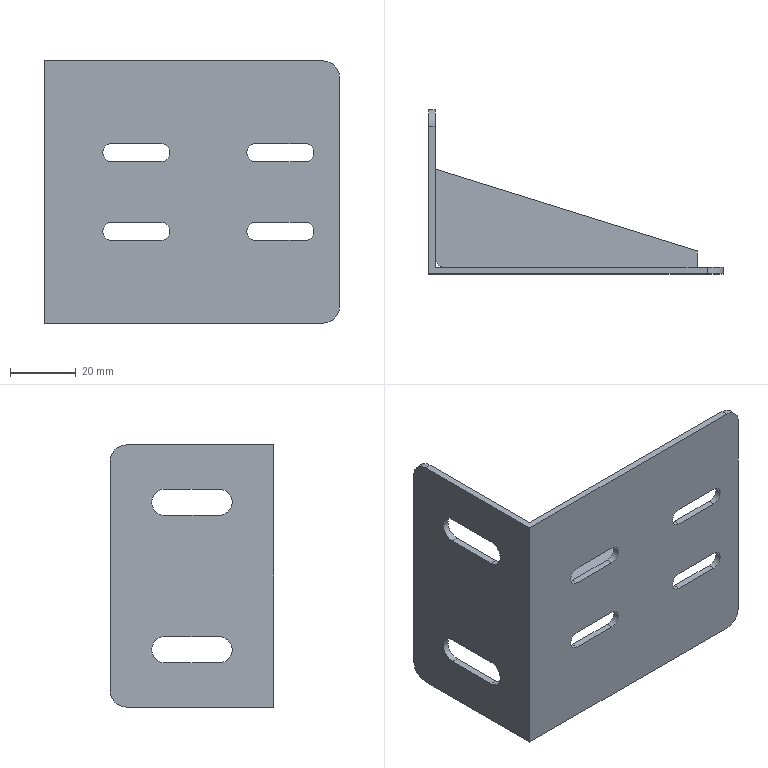Part | SolidWorks | features ICE 3, ExtruThin 1, Fillet 1 | 2 solids | 45 faces | box 90 x 50 x 80 mm | volume 23252 mm3 | plane 26 | cylinder 19 | commonest cylinder face diameters 5.5 x8 8 x6 10 x4 6 x1
STEP:
#1=CARTESIAN_POINT('',(2.,32.,-1.));
#2=VERTEX_POINT('',#1);
#3=CARTESIAN_POINT('',(2.,5.,-1.));
#4=VERTEX_POINT('',#3);
#5=CARTESIAN_POINT('',(2.,5.,-1.));
#6=DIRECTION('',(0.,-1.,0.));
#7=VECTOR('',#6,1000.);
#8=LINE('',#5,#7);
#9=EDGE_CURVE('',#2,#4,#8,.T.);
#10=ORIENTED_EDGE('',*,*,#9,.T.);
#11=CARTESIAN_POINT('',(2.,5.,1.));
#12=VERTEX_POINT('',#11);
#13=CARTESIAN_POINT('',(2.,5.,1.));
#14=DIRECTION('',(0.,0.,-1.));
#15=VECTOR('',#14,1000.);
#16=LINE('',#13,#15);
#17=EDGE_CURVE('',#12,#4,#16,.T.);
#18=ORIENTED_EDGE('',*,*,#17,.F.);
#19=CARTESIAN_POINT('',(2.,32.,1.));
#20=VERTEX_POINT('',#19);
#21=CARTESIAN_POINT('',(2.,5.,1.));
#22=DIRECTION('',(0.,-1.,0.));
#23=VECTOR('',#22,1000.);
#24=LINE('',#21,#23);
#25=EDGE_CURVE('',#20,#12,#24,.T.);
#26=ORIENTED_EDGE('',*,*,#25,.F.);
#27=CARTESIAN_POINT('',(2.,32.,1.));
#28=DIRECTION('',(0.,0.,-1.));
#29=VECTOR('',#28,1000.);
#30=LINE('',#27,#29);
#31=EDGE_CURVE('',#20,#2,#30,.T.);
#32=ORIENTED_EDGE('',*,*,#31,.T.);
#33=EDGE_LOOP('',(#10,#18,#26,#32));
#34=FACE_OUTER_BOUND('',#33,.T.);
#35=CARTESIAN_POINT('',(2.,5.,1.));
#36=DIRECTION('',(1.,0.,0.));
#37=DIRECTION('',(0.,1.,0.));
#38=AXIS2_PLACEMENT_3D('',#35,#36,#37);
#39=PLANE('',#38);
#40=ADVANCED_FACE('',(#34),#39,.F.);
#41=CARTESIAN_POINT('',(5.,2.,-1.));
#42=VERTEX_POINT('',#41);
#43=CARTESIAN_POINT('',(5.,5.,-1.));
#44=DIRECTION('',(0.,0.,1.));
#45=DIRECTION('',(-1.,0.,0.));
#46=AXIS2_PLACEMENT_3D('',#43,#44,#45);
#47=CIRCLE('',#46,3.);
#48=EDGE_CURVE('',#4,#42,#47,.T.);
#49=ORIENTED_EDGE('',*,*,#48,.T.);
#50=CARTESIAN_POINT('',(5.,2.,1.));
#51=VERTEX_POINT('',#50);
#52=CARTESIAN_POINT('',(5.,2.,1.));
#53=DIRECTION('',(0.,0.,-1.));
#54=VECTOR('',#53,1000.);
#55=LINE('',#52,#54);
#56=EDGE_CURVE('',#51,#42,#55,.T.);
#57=ORIENTED_EDGE('',*,*,#56,.F.);
#58=CARTESIAN_POINT('',(5.,5.,1.));
#59=DIRECTION('',(0.,0.,1.));
#60=DIRECTION('',(-1.,0.,0.));
#61=AXIS2_PLACEMENT_3D('',#58,#59,#60);
#62=CIRCLE('',#61,3.);
#63=EDGE_CURVE('',#12,#51,#62,.T.);
#64=ORIENTED_EDGE('',*,*,#63,.F.);
#65=ORIENTED_EDGE('',*,*,#17,.T.);
#66=EDGE_LOOP('',(#49,#57,#64,#65));
#67=FACE_OUTER_BOUND('',#66,.T.);
#68=CARTESIAN_POINT('',(5.,5.,1.));
#69=DIRECTION('',(0.,0.,-1.));
#70=DIRECTION('',(-1.,0.,0.));
#71=AXIS2_PLACEMENT_3D('',#68,#69,#70);
#72=CYLINDRICAL_SURFACE('',#71,3.);
#73=ADVANCED_FACE('',(#67),#72,.T.);
#74=CARTESIAN_POINT('',(82.,2.,-1.));
#75=VERTEX_POINT('',#74);
#76=CARTESIAN_POINT('',(82.,2.,-1.));
#77=DIRECTION('',(1.,0.,0.));
#78=VECTOR('',#77,1000.);
#79=LINE('',#76,#78);
#80=EDGE_CURVE('',#42,#75,#79,.T.);
#81=ORIENTED_EDGE('',*,*,#80,.T.);
#82=CARTESIAN_POINT('',(82.,2.,1.));
#83=VERTEX_POINT('',#82);
#84=CARTESIAN_POINT('',(82.,2.,1.));
#85=DIRECTION('',(0.,0.,-1.));
#86=VECTOR('',#85,1000.);
#87=LINE('',#84,#86);
#88=EDGE_CURVE('',#83,#75,#87,.T.);
#89=ORIENTED_EDGE('',*,*,#88,.F.);
#90=CARTESIAN_POINT('',(82.,2.,1.));
#91=DIRECTION('',(1.,0.,0.));
#92=VECTOR('',#91,1000.);
#93=LINE('',#90,#92);
#94=EDGE_CURVE('',#51,#83,#93,.T.);
#95=ORIENTED_EDGE('',*,*,#94,.F.);
#96=ORIENTED_EDGE('',*,*,#56,.T.);
#97=EDGE_LOOP('',(#81,#89,#95,#96));
#98=FACE_OUTER_BOUND('',#97,.T.);
#99=CARTESIAN_POINT('',(82.,2.,1.));
#100=DIRECTION('',(0.,1.,0.));
#101=DIRECTION('',(0.,0.,1.));
#102=AXIS2_PLACEMENT_3D('',#99,#100,#101);
#103=PLANE('',#102);
#104=ADVANCED_FACE('',(#98),#103,.F.);
#105=CARTESIAN_POINT('',(82.,7.,-1.));
#106=VERTEX_POINT('',#105);
#107=CARTESIAN_POINT('',(82.,7.,-1.));
#108=DIRECTION('',(0.,1.,0.));
#109=VECTOR('',#108,1000.);
#110=LINE('',#107,#109);
#111=EDGE_CURVE('',#75,#106,#110,.T.);
#112=ORIENTED_EDGE('',*,*,#111,.T.);
#113=CARTESIAN_POINT('',(82.,7.,1.));
#114=VERTEX_POINT('',#113);
#115=CARTESIAN_POINT('',(82.,7.,1.));
#116=DIRECTION('',(0.,0.,-1.));
#117=VECTOR('',#116,1000.);
#118=LINE('',#115,#117);
#119=EDGE_CURVE('',#114,#106,#118,.T.);
#120=ORIENTED_EDGE('',*,*,#119,.F.);
#121=CARTESIAN_POINT('',(82.,7.,1.));
#122=DIRECTION('',(0.,1.,0.));
#123=VECTOR('',#122,1000.);
#124=LINE('',#121,#123);
#125=EDGE_CURVE('',#83,#114,#124,.T.);
#126=ORIENTED_EDGE('',*,*,#125,.F.);
#127=ORIENTED_EDGE('',*,*,#88,.T.);
#128=EDGE_LOOP('',(#112,#120,#126,#127));
#129=FACE_OUTER_BOUND('',#128,.T.);
#130=CARTESIAN_POINT('',(82.,7.,1.));
#131=DIRECTION('',(-1.,0.,0.));
#132=DIRECTION('',(0.,0.,1.));
#133=AXIS2_PLACEMENT_3D('',#130,#131,#132);
#134=PLANE('',#133);
#135=ADVANCED_FACE('',(#129),#134,.F.);
#136=CARTESIAN_POINT('',(2.,32.,-1.));
#137=DIRECTION('',(-0.9545,0.2983,0.));
#138=VECTOR('',#137,1000.);
#139=LINE('',#136,#138);
#140=EDGE_CURVE('',#106,#2,#139,.T.);
#141=ORIENTED_EDGE('',*,*,#140,.T.);
#142=ORIENTED_EDGE('',*,*,#31,.F.);
#143=CARTESIAN_POINT('',(2.,32.,1.));
#144=DIRECTION('',(-0.9545,0.2983,0.));
#145=VECTOR('',#144,1000.);
#146=LINE('',#143,#145);
#147=EDGE_CURVE('',#114,#20,#146,.T.);
#148=ORIENTED_EDGE('',*,*,#147,.F.);
#149=ORIENTED_EDGE('',*,*,#119,.T.);
#150=EDGE_LOOP('',(#141,#142,#148,#149));
#151=FACE_OUTER_BOUND('',#150,.T.);
#152=CARTESIAN_POINT('',(2.,32.,1.));
#153=DIRECTION('',(-0.2983,-0.9545,0.));
#154=DIRECTION('',(0.9545,-0.2983,0.));
#155=AXIS2_PLACEMENT_3D('',#152,#153,#154);
#156=PLANE('',#155);
#157=ADVANCED_FACE('',(#151),#156,.F.);
#158=ORIENTED_EDGE('',*,*,#25,.T.);
#159=ORIENTED_EDGE('',*,*,#63,.T.);
#160=ORIENTED_EDGE('',*,*,#94,.T.);
#161=ORIENTED_EDGE('',*,*,#125,.T.);
#162=ORIENTED_EDGE('',*,*,#147,.T.);
#163=EDGE_LOOP('',(#158,#159,#160,#161,#162));
#164=FACE_OUTER_BOUND('',#163,.T.);
#165=CARTESIAN_POINT('',(5.,5.,1.));
#166=DIRECTION('',(0.,0.,-1.));
#167=DIRECTION('',(-1.,0.,0.));
#168=AXIS2_PLACEMENT_3D('',#165,#166,#167);
#169=PLANE('',#168);
#170=ADVANCED_FACE('',(#164),#169,.F.);
#171=ORIENTED_EDGE('',*,*,#9,.F.);
#172=ORIENTED_EDGE('',*,*,#140,.F.);
#173=ORIENTED_EDGE('',*,*,#111,.F.);
#174=ORIENTED_EDGE('',*,*,#80,.F.);
#175=ORIENTED_EDGE('',*,*,#48,.F.);
#176=EDGE_LOOP('',(#171,#172,#173,#174,#175));
#177=FACE_OUTER_BOUND('',#176,.T.);
#178=CARTESIAN_POINT('',(5.,5.,-1.));
#179=DIRECTION('',(0.,0.,-1.));
#180=DIRECTION('',(-1.,0.,0.));
#181=AXIS2_PLACEMENT_3D('',#178,#179,#180);
#182=PLANE('',#181);
#183=ADVANCED_FACE('',(#177),#182,.T.);
#184=CLOSED_SHELL('',(#40,#73,#104,#135,#157,#170,#183));
#185=MANIFOLD_SOLID_BREP('',#184);
#186=CARTESIAN_POINT('',(0.,37.284,22.5));
#187=VERTEX_POINT('',#186);
#188=CARTESIAN_POINT('',(0.,33.284,26.5));
#189=VERTEX_POINT('',#188);
#190=CARTESIAN_POINT('',(0.,33.284,22.5));
#191=DIRECTION('',(1.,0.,0.));
#192=DIRECTION('',(0.,1.,0.));
#193=AXIS2_PLACEMENT_3D('',#190,#191,#192);
#194=CIRCLE('',#193,4.);
#195=EDGE_CURVE('',#187,#189,#194,.T.);
#196=ORIENTED_EDGE('',*,*,#195,.F.);
#197=CARTESIAN_POINT('',(2.,37.284,22.5));
#198=VERTEX_POINT('',#197);
#199=CARTESIAN_POINT('',(0.,37.284,22.5));
#200=DIRECTION('',(1.,0.,0.));
#201=VECTOR('',#200,1000.);
#202=LINE('',#199,#201);
#203=EDGE_CURVE('',#187,#198,#202,.T.);
#204=ORIENTED_EDGE('',*,*,#203,.T.);
#205=CARTESIAN_POINT('',(2.,33.284,26.5));
#206=VERTEX_POINT('',#205);
#207=CARTESIAN_POINT('',(2.,33.284,22.5));
#208=DIRECTION('',(1.,0.,0.));
#209=DIRECTION('',(0.,1.,0.));
#210=AXIS2_PLACEMENT_3D('',#207,#208,#209);
#211=CIRCLE('',#210,4.);
#212=EDGE_CURVE('',#198,#206,#211,.T.);
#213=ORIENTED_EDGE('',*,*,#212,.T.);
#214=CARTESIAN_POINT('',(0.,33.284,26.5));
#215=DIRECTION('',(1.,0.,0.));
#216=VECTOR('',#215,1000.);
#217=LINE('',#214,#216);
#218=EDGE_CURVE('',#189,#206,#217,.T.);
#219=ORIENTED_EDGE('',*,*,#218,.F.);
#220=EDGE_LOOP('',(#196,#204,#213,#219));
#221=FACE_OUTER_BOUND('',#220,.T.);
#222=CARTESIAN_POINT('',(0.,33.284,22.5));
#223=DIRECTION('',(1.,0.,0.));
#224=DIRECTION('',(0.,1.,0.));
#225=AXIS2_PLACEMENT_3D('',#222,#223,#224);
#226=CYLINDRICAL_SURFACE('',#225,4.);
#227=ADVANCED_FACE('',(#221),#226,.F.);
#228=CARTESIAN_POINT('',(0.,37.284,-22.5));
#229=VERTEX_POINT('',#228);
#230=CARTESIAN_POINT('',(0.,33.284,-18.5));
#231=VERTEX_POINT('',#230);
#232=CARTESIAN_POINT('',(0.,33.284,-22.5));
#233=DIRECTION('',(1.,0.,0.));
#234=DIRECTION('',(0.,-1.,0.));
#235=AXIS2_PLACEMENT_3D('',#232,#233,#234);
#236=CIRCLE('',#235,4.);
#237=EDGE_CURVE('',#229,#231,#236,.T.);
#238=ORIENTED_EDGE('',*,*,#237,.F.);
#239=CARTESIAN_POINT('',(2.,37.284,-22.5));
#240=VERTEX_POINT('',#239);
#241=CARTESIAN_POINT('',(0.,37.284,-22.5));
#242=DIRECTION('',(1.,0.,0.));
#243=VECTOR('',#242,1000.);
#244=LINE('',#241,#243);
#245=EDGE_CURVE('',#229,#240,#244,.T.);
#246=ORIENTED_EDGE('',*,*,#245,.T.);
#247=CARTESIAN_POINT('',(2.,33.284,-18.5));
#248=VERTEX_POINT('',#247);
#249=CARTESIAN_POINT('',(2.,33.284,-22.5));
#250=DIRECTION('',(1.,0.,0.));
#251=DIRECTION('',(0.,-1.,0.));
#252=AXIS2_PLACEMENT_3D('',#249,#250,#251);
#253=CIRCLE('',#252,4.);
#254=EDGE_CURVE('',#240,#248,#253,.T.);
#255=ORIENTED_EDGE('',*,*,#254,.T.);
#256=CARTESIAN_POINT('',(0.,33.284,-18.5));
#257=DIRECTION('',(1.,0.,0.));
#258=VECTOR('',#257,1000.);
#259=LINE('',#256,#258);
#260=EDGE_CURVE('',#231,#248,#259,.T.);
#261=ORIENTED_EDGE('',*,*,#260,.F.);
#262=EDGE_LOOP('',(#238,#246,#255,#261));
#263=FACE_OUTER_BOUND('',#262,.T.);
#264=CARTESIAN_POINT('',(0.,33.284,-22.5));
#265=DIRECTION('',(1.,0.,0.));
#266=DIRECTION('',(0.,1.,0.));
#267=AXIS2_PLACEMENT_3D('',#264,#265,#266);
#268=CYLINDRICAL_SURFACE('',#267,4.);
#269=ADVANCED_FACE('',(#263),#268,.F.);
#270=CARTESIAN_POINT('',(64.5,0.,9.25));
#271=VERTEX_POINT('',#270);
#272=CARTESIAN_POINT('',(64.5,0.,14.75));
#273=VERTEX_POINT('',#272);
#274=CARTESIAN_POINT('',(64.5,0.,12.));
#275=DIRECTION('',(0.,1.,0.));
#276=DIRECTION('',(0.,0.,1.));
#277=AXIS2_PLACEMENT_3D('',#274,#275,#276);
#278=CIRCLE('',#277,2.75);
#279=EDGE_CURVE('',#271,#273,#278,.T.);
#280=ORIENTED_EDGE('',*,*,#279,.T.);
#281=CARTESIAN_POINT('',(79.5,0.,14.75));
#282=VERTEX_POINT('',#281);
#283=CARTESIAN_POINT('',(64.5,0.,14.75));
#284=DIRECTION('',(1.,0.,0.));
#285=VECTOR('',#284,1000.);
#286=LINE('',#283,#285);
#287=EDGE_CURVE('',#273,#282,#286,.T.);
#288=ORIENTED_EDGE('',*,*,#287,.T.);
#289=CARTESIAN_POINT('',(79.5,0.,9.25));
#290=VERTEX_POINT('',#289);
#291=CARTESIAN_POINT('',(79.5,0.,12.));
#292=DIRECTION('',(0.,1.,0.));
#293=DIRECTION('',(0.,0.,1.));
#294=AXIS2_PLACEMENT_3D('',#291,#292,#293);
#295=CIRCLE('',#294,2.75);
#296=EDGE_CURVE('',#282,#290,#295,.T.);
#297=ORIENTED_EDGE('',*,*,#296,.T.);
#298=CARTESIAN_POINT('',(64.5,0.,9.25));
#299=DIRECTION('',(-1.,0.,0.));
#300=VECTOR('',#299,1000.);
#301=LINE('',#298,#300);
#302=EDGE_CURVE('',#290,#271,#301,.T.);
#303=ORIENTED_EDGE('',*,*,#302,.T.);
#304=EDGE_LOOP('',(#280,#288,#297,#303));
#305=FACE_BOUND('',#304,.T.);
#306=CARTESIAN_POINT('',(20.5,0.,-14.75));
#307=VERTEX_POINT('',#306);
#308=CARTESIAN_POINT('',(20.5,0.,-9.25));
#309=VERTEX_POINT('',#308);
#310=CARTESIAN_POINT('',(20.5,0.,-12.));
#311=DIRECTION('',(0.,1.,0.));
#312=DIRECTION('',(0.,0.,1.));
#313=AXIS2_PLACEMENT_3D('',#310,#311,#312);
#314=CIRCLE('',#313,2.75);
#315=EDGE_CURVE('',#307,#309,#314,.T.);
#316=ORIENTED_EDGE('',*,*,#315,.T.);
#317=CARTESIAN_POINT('',(35.5,0.,-9.25));
#318=VERTEX_POINT('',#317);
#319=CARTESIAN_POINT('',(20.5,0.,-9.25));
#320=DIRECTION('',(1.,0.,0.));
#321=VECTOR('',#320,1000.);
#322=LINE('',#319,#321);
#323=EDGE_CURVE('',#309,#318,#322,.T.);
#324=ORIENTED_EDGE('',*,*,#323,.T.);
#325=CARTESIAN_POINT('',(35.5,0.,-14.75));
#326=VERTEX_POINT('',#325);
#327=CARTESIAN_POINT('',(35.5,0.,-12.));
#328=DIRECTION('',(0.,1.,0.));
#329=DIRECTION('',(0.,0.,1.));
#330=AXIS2_PLACEMENT_3D('',#327,#328,#329);
#331=CIRCLE('',#330,2.75);
#332=EDGE_CURVE('',#318,#326,#331,.T.);
#333=ORIENTED_EDGE('',*,*,#332,.T.);
#334=CARTESIAN_POINT('',(20.5,0.,-14.75));
#335=DIRECTION('',(-1.,0.,0.));
#336=VECTOR('',#335,1000.);
#337=LINE('',#334,#336);
#338=EDGE_CURVE('',#326,#307,#337,.T.);
#339=ORIENTED_EDGE('',*,*,#338,.T.);
#340=EDGE_LOOP('',(#316,#324,#333,#339));
#341=FACE_BOUND('',#340,.T.);
#342=CARTESIAN_POINT('',(0.,0.,-40.));
#343=VERTEX_POINT('',#342);
#344=CARTESIAN_POINT('',(85.,0.,-40.));
#345=VERTEX_POINT('',#344);
#346=CARTESIAN_POINT('',(0.,0.,-40.));
#347=DIRECTION('',(1.,0.,0.));
#348=VECTOR('',#347,1000.);
#349=LINE('',#346,#348);
#350=EDGE_CURVE('',#343,#345,#349,.T.);
#351=ORIENTED_EDGE('',*,*,#350,.T.);
#352=CARTESIAN_POINT('',(90.,0.,-35.));
#353=VERTEX_POINT('',#352);
#354=CARTESIAN_POINT('',(85.,0.,-35.));
#355=DIRECTION('',(0.,-1.,0.));
#356=DIRECTION('',(0.,0.,1.));
#357=AXIS2_PLACEMENT_3D('',#354,#355,#356);
#358=CIRCLE('',#357,5.);
#359=EDGE_CURVE('',#345,#353,#358,.T.);
#360=ORIENTED_EDGE('',*,*,#359,.T.);
#361=CARTESIAN_POINT('',(90.,0.,35.));
#362=VERTEX_POINT('',#361);
#363=CARTESIAN_POINT('',(90.,0.,40.));
#364=DIRECTION('',(0.,0.,-1.));
#365=VECTOR('',#364,1000.);
#366=LINE('',#363,#365);
#367=EDGE_CURVE('',#362,#353,#366,.T.);
#368=ORIENTED_EDGE('',*,*,#367,.F.);
#369=CARTESIAN_POINT('',(85.,0.,40.));
#370=VERTEX_POINT('',#369);
#371=CARTESIAN_POINT('',(85.,0.,35.));
#372=DIRECTION('',(0.,-1.,0.));
#373=DIRECTION('',(0.,0.,1.));
#374=AXIS2_PLACEMENT_3D('',#371,#372,#373);
#375=CIRCLE('',#374,5.);
#376=EDGE_CURVE('',#362,#370,#375,.T.);
#377=ORIENTED_EDGE('',*,*,#376,.T.);
#378=CARTESIAN_POINT('',(0.,0.,40.));
#379=VERTEX_POINT('',#378);
#380=CARTESIAN_POINT('',(0.,0.,40.));
#381=DIRECTION('',(1.,0.,0.));
#382=VECTOR('',#381,1000.);
#383=LINE('',#380,#382);
#384=EDGE_CURVE('',#379,#370,#383,.T.);
#385=ORIENTED_EDGE('',*,*,#384,.F.);
#386=CARTESIAN_POINT('',(0.,0.,40.));
#387=DIRECTION('',(0.,0.,-1.));
#388=VECTOR('',#387,1000.);
#389=LINE('',#386,#388);
#390=EDGE_CURVE('',#379,#343,#389,.T.);
#391=ORIENTED_EDGE('',*,*,#390,.T.);
#392=EDGE_LOOP('',(#351,#360,#368,#377,#385,#391));
#393=FACE_OUTER_BOUND('',#392,.T.);
#394=CARTESIAN_POINT('',(64.5,0.,-14.75));
#395=VERTEX_POINT('',#394);
#396=CARTESIAN_POINT('',(64.5,0.,-9.25));
#397=VERTEX_POINT('',#396);
#398=CARTESIAN_POINT('',(64.5,0.,-12.));
#399=DIRECTION('',(0.,1.,0.));
#400=DIRECTION('',(0.,0.,1.));
#401=AXIS2_PLACEMENT_3D('',#398,#399,#400);
#402=CIRCLE('',#401,2.75);
#403=EDGE_CURVE('',#395,#397,#402,.T.);
#404=ORIENTED_EDGE('',*,*,#403,.T.);
#405=CARTESIAN_POINT('',(79.5,0.,-9.25));
#406=VERTEX_POINT('',#405);
#407=CARTESIAN_POINT('',(64.5,0.,-9.25));
#408=DIRECTION('',(1.,0.,0.));
#409=VECTOR('',#408,1000.);
#410=LINE('',#407,#409);
#411=EDGE_CURVE('',#397,#406,#410,.T.);
#412=ORIENTED_EDGE('',*,*,#411,.T.);
#413=CARTESIAN_POINT('',(79.5,0.,-14.75));
#414=VERTEX_POINT('',#413);
#415=CARTESIAN_POINT('',(79.5,0.,-12.));
#416=DIRECTION('',(0.,1.,0.));
#417=DIRECTION('',(0.,0.,1.));
#418=AXIS2_PLACEMENT_3D('',#415,#416,#417);
#419=CIRCLE('',#418,2.75);
#420=EDGE_CURVE('',#406,#414,#419,.T.);
#421=ORIENTED_EDGE('',*,*,#420,.T.);
#422=CARTESIAN_POINT('',(64.5,0.,-14.75));
#423=DIRECTION('',(-1.,0.,0.));
#424=VECTOR('',#423,1000.);
#425=LINE('',#422,#424);
#426=EDGE_CURVE('',#414,#395,#425,.T.);
#427=ORIENTED_EDGE('',*,*,#426,.T.);
#428=EDGE_LOOP('',(#404,#412,#421,#427));
#429=FACE_BOUND('',#428,.T.);
#430=CARTESIAN_POINT('',(20.5,0.,9.25));
#431=VERTEX_POINT('',#430);
#432=CARTESIAN_POINT('',(20.5,0.,14.75));
#433=VERTEX_POINT('',#432);
#434=CARTESIAN_POINT('',(20.5,0.,12.));
#435=DIRECTION('',(0.,1.,0.));
#436=DIRECTION('',(0.,0.,1.));
#437=AXIS2_PLACEMENT_3D('',#434,#435,#436);
#438=CIRCLE('',#437,2.75);
#439=EDGE_CURVE('',#431,#433,#438,.T.);
#440=ORIENTED_EDGE('',*,*,#439,.T.);
#441=CARTESIAN_POINT('',(35.5,0.,14.75));
#442=VERTEX_POINT('',#441);
#443=CARTESIAN_POINT('',(20.5,0.,14.75));
#444=DIRECTION('',(1.,0.,0.));
#445=VECTOR('',#444,1000.);
#446=LINE('',#443,#445);
#447=EDGE_CURVE('',#433,#442,#446,.T.);
#448=ORIENTED_EDGE('',*,*,#447,.T.);
#449=CARTESIAN_POINT('',(35.5,0.,9.25));
#450=VERTEX_POINT('',#449);
#451=CARTESIAN_POINT('',(35.5,0.,12.));
#452=DIRECTION('',(0.,1.,0.));
#453=DIRECTION('',(0.,0.,1.));
#454=AXIS2_PLACEMENT_3D('',#451,#452,#453);
#455=CIRCLE('',#454,2.75);
#456=EDGE_CURVE('',#442,#450,#455,.T.);
#457=ORIENTED_EDGE('',*,*,#456,.T.);
#458=CARTESIAN_POINT('',(20.5,0.,9.25));
#459=DIRECTION('',(-1.,0.,0.));
#460=VECTOR('',#459,1000.);
#461=LINE('',#458,#460);
#462=EDGE_CURVE('',#450,#431,#461,.T.);
#463=ORIENTED_EDGE('',*,*,#462,.T.);
#464=EDGE_LOOP('',(#440,#448,#457,#463));
#465=FACE_BOUND('',#464,.T.);
#466=CARTESIAN_POINT('',(0.,0.,40.));
#467=DIRECTION('',(0.,1.,0.));
#468=DIRECTION('',(0.,0.,1.));
#469=AXIS2_PLACEMENT_3D('',#466,#467,#468);
#470=PLANE('',#469);
#471=ADVANCED_FACE('',(#305,#341,#393,#429,#465),#470,.F.);
#472=CARTESIAN_POINT('',(90.,2.,35.));
#473=VERTEX_POINT('',#472);
#474=CARTESIAN_POINT('',(90.,2.,-35.));
#475=VERTEX_POINT('',#474);
#476=CARTESIAN_POINT('',(90.,2.,40.));
#477=DIRECTION('',(0.,0.,-1.));
#478=VECTOR('',#477,1000.);
#479=LINE('',#476,#478);
#480=EDGE_CURVE('',#473,#475,#479,.T.);
#481=ORIENTED_EDGE('',*,*,#480,.T.);
#482=CARTESIAN_POINT('',(85.,2.,-40.));
#483=VERTEX_POINT('',#482);
#484=CARTESIAN_POINT('',(85.,2.,-35.));
#485=DIRECTION('',(0.,1.,0.));
#486=DIRECTION('',(0.,0.,1.));
#487=AXIS2_PLACEMENT_3D('',#484,#485,#486);
#488=CIRCLE('',#487,5.);
#489=EDGE_CURVE('',#475,#483,#488,.T.);
#490=ORIENTED_EDGE('',*,*,#489,.T.);
#491=CARTESIAN_POINT('',(2.,2.,-40.));
#492=VERTEX_POINT('',#491);
#493=CARTESIAN_POINT('',(0.,2.,-40.));
#494=DIRECTION('',(1.,0.,0.));
#495=VECTOR('',#494,1000.);
#496=LINE('',#493,#495);
#497=EDGE_CURVE('',#492,#483,#496,.T.);
#498=ORIENTED_EDGE('',*,*,#497,.F.);
#499=CARTESIAN_POINT('',(2.,2.,40.));
#500=VERTEX_POINT('',#499);
#501=CARTESIAN_POINT('',(2.,2.,40.));
#502=DIRECTION('',(0.,0.,-1.));
#503=VECTOR('',#502,1000.);
#504=LINE('',#501,#503);
#505=EDGE_CURVE('',#500,#492,#504,.T.);
#506=ORIENTED_EDGE('',*,*,#505,.F.);
#507=CARTESIAN_POINT('',(85.,2.,40.));
#508=VERTEX_POINT('',#507);
#509=CARTESIAN_POINT('',(0.,2.,40.));
#510=DIRECTION('',(1.,0.,0.));
#511=VECTOR('',#510,1000.);
#512=LINE('',#509,#511);
#513=EDGE_CURVE('',#500,#508,#512,.T.);
#514=ORIENTED_EDGE('',*,*,#513,.T.);
#515=CARTESIAN_POINT('',(85.,2.,35.));
#516=DIRECTION('',(0.,1.,0.));
#517=DIRECTION('',(0.,0.,1.));
#518=AXIS2_PLACEMENT_3D('',#515,#516,#517);
#519=CIRCLE('',#518,5.);
#520=EDGE_CURVE('',#508,#473,#519,.T.);
#521=ORIENTED_EDGE('',*,*,#520,.T.);
#522=EDGE_LOOP('',(#481,#490,#498,#506,#514,#521));
#523=FACE_OUTER_BOUND('',#522,.T.);
#524=CARTESIAN_POINT('',(35.5,2.,-9.25));
#525=VERTEX_POINT('',#524);
#526=CARTESIAN_POINT('',(20.5,2.,-9.25));
#527=VERTEX_POINT('',#526);
#528=CARTESIAN_POINT('',(0.,2.,-9.25));
#529=DIRECTION('',(-1.,0.,0.));
#530=VECTOR('',#529,1000.);
#531=LINE('',#528,#530);
#532=EDGE_CURVE('',#525,#527,#531,.T.);
#533=ORIENTED_EDGE('',*,*,#532,.T.);
#534=CARTESIAN_POINT('',(20.5,2.,-14.75));
#535=VERTEX_POINT('',#534);
#536=CARTESIAN_POINT('',(20.5,2.,-12.));
#537=DIRECTION('',(0.,-1.,0.));
#538=DIRECTION('',(0.,0.,1.));
#539=AXIS2_PLACEMENT_3D('',#536,#537,#538);
#540=CIRCLE('',#539,2.75);
#541=EDGE_CURVE('',#527,#535,#540,.T.);
#542=ORIENTED_EDGE('',*,*,#541,.T.);
#543=CARTESIAN_POINT('',(35.5,2.,-14.75));
#544=VERTEX_POINT('',#543);
#545=CARTESIAN_POINT('',(0.,2.,-14.75));
#546=DIRECTION('',(1.,0.,0.));
#547=VECTOR('',#546,1000.);
#548=LINE('',#545,#547);
#549=EDGE_CURVE('',#535,#544,#548,.T.);
#550=ORIENTED_EDGE('',*,*,#549,.T.);
#551=CARTESIAN_POINT('',(35.5,2.,-12.));
#552=DIRECTION('',(0.,-1.,0.));
#553=DIRECTION('',(0.,0.,1.));
#554=AXIS2_PLACEMENT_3D('',#551,#552,#553);
#555=CIRCLE('',#554,2.75);
#556=EDGE_CURVE('',#544,#525,#555,.T.);
#557=ORIENTED_EDGE('',*,*,#556,.T.);
#558=EDGE_LOOP('',(#533,#542,#550,#557));
#559=FACE_BOUND('',#558,.T.);
#560=CARTESIAN_POINT('',(79.5,2.,-9.25));
#561=VERTEX_POINT('',#560);
#562=CARTESIAN_POINT('',(64.5,2.,-9.25));
#563=VERTEX_POINT('',#562);
#564=CARTESIAN_POINT('',(0.,2.,-9.25));
#565=DIRECTION('',(-1.,0.,0.));
#566=VECTOR('',#565,1000.);
#567=LINE('',#564,#566);
#568=EDGE_CURVE('',#561,#563,#567,.T.);
#569=ORIENTED_EDGE('',*,*,#568,.T.);
#570=CARTESIAN_POINT('',(64.5,2.,-14.75));
#571=VERTEX_POINT('',#570);
#572=CARTESIAN_POINT('',(64.5,2.,-12.));
#573=DIRECTION('',(0.,-1.,0.));
#574=DIRECTION('',(0.,0.,1.));
#575=AXIS2_PLACEMENT_3D('',#572,#573,#574);
#576=CIRCLE('',#575,2.75);
#577=EDGE_CURVE('',#563,#571,#576,.T.);
#578=ORIENTED_EDGE('',*,*,#577,.T.);
#579=CARTESIAN_POINT('',(79.5,2.,-14.75));
#580=VERTEX_POINT('',#579);
#581=CARTESIAN_POINT('',(0.,2.,-14.75));
#582=DIRECTION('',(1.,0.,0.));
#583=VECTOR('',#582,1000.);
#584=LINE('',#581,#583);
#585=EDGE_CURVE('',#571,#580,#584,.T.);
#586=ORIENTED_EDGE('',*,*,#585,.T.);
#587=CARTESIAN_POINT('',(79.5,2.,-12.));
#588=DIRECTION('',(0.,-1.,0.));
#589=DIRECTION('',(0.,0.,1.));
#590=AXIS2_PLACEMENT_3D('',#587,#588,#589);
#591=CIRCLE('',#590,2.75);
#592=EDGE_CURVE('',#580,#561,#591,.T.);
#593=ORIENTED_EDGE('',*,*,#592,.T.);
#594=EDGE_LOOP('',(#569,#578,#586,#593));
#595=FACE_BOUND('',#594,.T.);
#596=CARTESIAN_POINT('',(79.5,2.,14.75));
#597=VERTEX_POINT('',#596);
#598=CARTESIAN_POINT('',(64.5,2.,14.75));
#599=VERTEX_POINT('',#598);
#600=CARTESIAN_POINT('',(0.,2.,14.75));
#601=DIRECTION('',(-1.,0.,0.));
#602=VECTOR('',#601,1000.);
#603=LINE('',#600,#602);
#604=EDGE_CURVE('',#597,#599,#603,.T.);
#605=ORIENTED_EDGE('',*,*,#604,.T.);
#606=CARTESIAN_POINT('',(64.5,2.,9.25));
#607=VERTEX_POINT('',#606);
#608=CARTESIAN_POINT('',(64.5,2.,12.));
#609=DIRECTION('',(0.,-1.,0.));
#610=DIRECTION('',(0.,0.,1.));
#611=AXIS2_PLACEMENT_3D('',#608,#609,#610);
#612=CIRCLE('',#611,2.75);
#613=EDGE_CURVE('',#599,#607,#612,.T.);
#614=ORIENTED_EDGE('',*,*,#613,.T.);
#615=CARTESIAN_POINT('',(79.5,2.,9.25));
#616=VERTEX_POINT('',#615);
#617=CARTESIAN_POINT('',(0.,2.,9.25));
#618=DIRECTION('',(1.,0.,0.));
#619=VECTOR('',#618,1000.);
#620=LINE('',#617,#619);
#621=EDGE_CURVE('',#607,#616,#620,.T.);
#622=ORIENTED_EDGE('',*,*,#621,.T.);
#623=CARTESIAN_POINT('',(79.5,2.,12.));
#624=DIRECTION('',(0.,-1.,0.));
#625=DIRECTION('',(0.,0.,1.));
#626=AXIS2_PLACEMENT_3D('',#623,#624,#625);
#627=CIRCLE('',#626,2.75);
#628=EDGE_CURVE('',#616,#597,#627,.T.);
#629=ORIENTED_EDGE('',*,*,#628,.T.);
#630=EDGE_LOOP('',(#605,#614,#622,#629));
#631=FACE_BOUND('',#630,.T.);
#632=CARTESIAN_POINT('',(35.5,2.,14.75));
#633=VERTEX_POINT('',#632);
#634=CARTESIAN_POINT('',(20.5,2.,14.75));
#635=VERTEX_POINT('',#634);
#636=CARTESIAN_POINT('',(0.,2.,14.75));
#637=DIRECTION('',(-1.,0.,0.));
#638=VECTOR('',#637,1000.);
#639=LINE('',#636,#638);
#640=EDGE_CURVE('',#633,#635,#639,.T.);
#641=ORIENTED_EDGE('',*,*,#640,.T.);
#642=CARTESIAN_POINT('',(20.5,2.,9.25));
#643=VERTEX_POINT('',#642);
#644=CARTESIAN_POINT('',(20.5,2.,12.));
#645=DIRECTION('',(0.,-1.,0.));
#646=DIRECTION('',(0.,0.,1.));
#647=AXIS2_PLACEMENT_3D('',#644,#645,#646);
#648=CIRCLE('',#647,2.75);
#649=EDGE_CURVE('',#635,#643,#648,.T.);
#650=ORIENTED_EDGE('',*,*,#649,.T.);
#651=CARTESIAN_POINT('',(35.5,2.,9.25));
#652=VERTEX_POINT('',#651);
#653=CARTESIAN_POINT('',(0.,2.,9.25));
#654=DIRECTION('',(1.,0.,0.));
#655=VECTOR('',#654,1000.);
#656=LINE('',#653,#655);
#657=EDGE_CURVE('',#643,#652,#656,.T.);
#658=ORIENTED_EDGE('',*,*,#657,.T.);
#659=CARTESIAN_POINT('',(35.5,2.,12.));
#660=DIRECTION('',(0.,-1.,0.));
#661=DIRECTION('',(0.,0.,1.));
#662=AXIS2_PLACEMENT_3D('',#659,#660,#661);
#663=CIRCLE('',#662,2.75);
#664=EDGE_CURVE('',#652,#633,#663,.T.);
#665=ORIENTED_EDGE('',*,*,#664,.T.);
#666=EDGE_LOOP('',(#641,#650,#658,#665));
#667=FACE_BOUND('',#666,.T.);
#668=CARTESIAN_POINT('',(0.,2.,40.));
#669=DIRECTION('',(0.,1.,0.));
#670=DIRECTION('',(0.,0.,1.));
#671=AXIS2_PLACEMENT_3D('',#668,#669,#670);
#672=PLANE('',#671);
#673=ADVANCED_FACE('',(#523,#559,#595,#631,#667),#672,.T.);
#674=ORIENTED_EDGE('',*,*,#367,.T.);
#675=CARTESIAN_POINT('',(90.,2.,-35.));
#676=DIRECTION('',(0.,1.,0.));
#677=VECTOR('',#676,1000.);
#678=LINE('',#675,#677);
#679=EDGE_CURVE('',#353,#475,#678,.T.);
#680=ORIENTED_EDGE('',*,*,#679,.T.);
#681=ORIENTED_EDGE('',*,*,#480,.F.);
#682=CARTESIAN_POINT('',(90.,0.,35.));
#683=DIRECTION('',(0.,-1.,0.));
#684=VECTOR('',#683,1000.);
#685=LINE('',#682,#684);
#686=EDGE_CURVE('',#473,#362,#685,.T.);
#687=ORIENTED_EDGE('',*,*,#686,.T.);
#688=EDGE_LOOP('',(#674,#680,#681,#687));
#689=FACE_OUTER_BOUND('',#688,.T.);
#690=CARTESIAN_POINT('',(90.,2.,40.));
#691=DIRECTION('',(1.,0.,0.));
#692=DIRECTION('',(0.,0.,-1.));
#693=AXIS2_PLACEMENT_3D('',#690,#691,#692);
#694=PLANE('',#693);
#695=ADVANCED_FACE('',(#689),#694,.T.);
#696=CARTESIAN_POINT('',(2.,33.284,18.5));
#697=VERTEX_POINT('',#696);
#698=CARTESIAN_POINT('',(2.,33.284,22.5));
#699=DIRECTION('',(1.,0.,0.));
#700=DIRECTION('',(0.,1.,0.));
#701=AXIS2_PLACEMENT_3D('',#698,#699,#700);
#702=CIRCLE('',#701,4.);
#703=EDGE_CURVE('',#697,#198,#702,.T.);
#704=ORIENTED_EDGE('',*,*,#703,.F.);
#705=CARTESIAN_POINT('',(2.,16.716,18.5));
#706=VERTEX_POINT('',#705);
#707=CARTESIAN_POINT('',(2.,33.284,18.5));
#708=DIRECTION('',(0.,1.,0.));
#709=VECTOR('',#708,1000.);
#710=LINE('',#707,#709);
#711=EDGE_CURVE('',#706,#697,#710,.T.);
#712=ORIENTED_EDGE('',*,*,#711,.F.);
#713=CARTESIAN_POINT('',(2.,16.716,26.5));
#714=VERTEX_POINT('',#713);
#715=CARTESIAN_POINT('',(2.,16.716,22.5));
#716=DIRECTION('',(1.,0.,0.));
#717=DIRECTION('',(0.,1.,0.));
#718=AXIS2_PLACEMENT_3D('',#715,#716,#717);
#719=CIRCLE('',#718,4.);
#720=EDGE_CURVE('',#714,#706,#719,.T.);
#721=ORIENTED_EDGE('',*,*,#720,.F.);
#722=CARTESIAN_POINT('',(2.,33.284,26.5));
#723=DIRECTION('',(0.,-1.,0.));
#724=VECTOR('',#723,1000.);
#725=LINE('',#722,#724);
#726=EDGE_CURVE('',#206,#714,#725,.T.);
#727=ORIENTED_EDGE('',*,*,#726,.F.);
#728=ORIENTED_EDGE('',*,*,#212,.F.);
#729=EDGE_LOOP('',(#704,#712,#721,#727,#728));
#730=FACE_BOUND('',#729,.T.);
#731=CARTESIAN_POINT('',(2.,33.284,-26.5));
#732=VERTEX_POINT('',#731);
#733=CARTESIAN_POINT('',(2.,33.284,-22.5));
#734=DIRECTION('',(1.,0.,0.));
#735=DIRECTION('',(0.,-1.,0.));
#736=AXIS2_PLACEMENT_3D('',#733,#734,#735);
#737=CIRCLE('',#736,4.);
#738=EDGE_CURVE('',#732,#240,#737,.T.);
#739=ORIENTED_EDGE('',*,*,#738,.F.);
#740=CARTESIAN_POINT('',(2.,16.716,-26.5));
#741=VERTEX_POINT('',#740);
#742=CARTESIAN_POINT('',(2.,33.284,-26.5));
#743=DIRECTION('',(0.,1.,0.));
#744=VECTOR('',#743,1000.);
#745=LINE('',#742,#744);
#746=EDGE_CURVE('',#741,#732,#745,.T.);
#747=ORIENTED_EDGE('',*,*,#746,.F.);
#748=CARTESIAN_POINT('',(2.,16.716,-18.5));
#749=VERTEX_POINT('',#748);
#750=CARTESIAN_POINT('',(2.,16.716,-22.5));
#751=DIRECTION('',(1.,0.,0.));
#752=DIRECTION('',(0.,-1.,0.));
#753=AXIS2_PLACEMENT_3D('',#750,#751,#752);
#754=CIRCLE('',#753,4.);
#755=EDGE_CURVE('',#749,#741,#754,.T.);
#756=ORIENTED_EDGE('',*,*,#755,.F.);
#757=CARTESIAN_POINT('',(2.,33.284,-18.5));
#758=DIRECTION('',(0.,-1.,0.));
#759=VECTOR('',#758,1000.);
#760=LINE('',#757,#759);
#761=EDGE_CURVE('',#248,#749,#760,.T.);
#762=ORIENTED_EDGE('',*,*,#761,.F.);
#763=ORIENTED_EDGE('',*,*,#254,.F.);
#764=EDGE_LOOP('',(#739,#747,#756,#762,#763));
#765=FACE_BOUND('',#764,.T.);
#766=CARTESIAN_POINT('',(2.,45.,-40.));
#767=VERTEX_POINT('',#766);
#768=CARTESIAN_POINT('',(2.,50.,-40.));
#769=DIRECTION('',(0.,-1.,0.));
#770=VECTOR('',#769,1000.);
#771=LINE('',#768,#770);
#772=EDGE_CURVE('',#767,#492,#771,.T.);
#773=ORIENTED_EDGE('',*,*,#772,.F.);
#774=CARTESIAN_POINT('',(2.,50.,-35.));
#775=VERTEX_POINT('',#774);
#776=CARTESIAN_POINT('',(2.,45.,-35.));
#777=DIRECTION('',(1.,0.,0.));
#778=DIRECTION('',(0.,1.,0.));
#779=AXIS2_PLACEMENT_3D('',#776,#777,#778);
#780=CIRCLE('',#779,5.);
#781=EDGE_CURVE('',#767,#775,#780,.T.);
#782=ORIENTED_EDGE('',*,*,#781,.T.);
#783=CARTESIAN_POINT('',(2.,50.,35.));
#784=VERTEX_POINT('',#783);
#785=CARTESIAN_POINT('',(2.,50.,40.));
#786=DIRECTION('',(0.,0.,-1.));
#787=VECTOR('',#786,1000.);
#788=LINE('',#785,#787);
#789=EDGE_CURVE('',#784,#775,#788,.T.);
#790=ORIENTED_EDGE('',*,*,#789,.F.);
#791=CARTESIAN_POINT('',(2.,45.,40.));
#792=VERTEX_POINT('',#791);
#793=CARTESIAN_POINT('',(2.,45.,35.));
#794=DIRECTION('',(1.,0.,0.));
#795=DIRECTION('',(0.,1.,0.));
#796=AXIS2_PLACEMENT_3D('',#793,#794,#795);
#797=CIRCLE('',#796,5.);
#798=EDGE_CURVE('',#784,#792,#797,.T.);
#799=ORIENTED_EDGE('',*,*,#798,.T.);
#800=CARTESIAN_POINT('',(2.,50.,40.));
#801=DIRECTION('',(0.,-1.,0.));
#802=VECTOR('',#801,1000.);
#803=LINE('',#800,#802);
#804=EDGE_CURVE('',#792,#500,#803,.T.);
#805=ORIENTED_EDGE('',*,*,#804,.T.);
#806=ORIENTED_EDGE('',*,*,#505,.T.);
#807=EDGE_LOOP('',(#773,#782,#790,#799,#805,#806));
#808=FACE_OUTER_BOUND('',#807,.T.);
#809=CARTESIAN_POINT('',(2.,50.,40.));
#810=DIRECTION('',(1.,0.,0.));
#811=DIRECTION('',(0.,1.,0.));
#812=AXIS2_PLACEMENT_3D('',#809,#810,#811);
#813=PLANE('',#812);
#814=ADVANCED_FACE('',(#730,#765,#808),#813,.T.);
#815=ORIENTED_EDGE('',*,*,#789,.T.);
#816=CARTESIAN_POINT('',(0.,50.,-35.));
#817=VERTEX_POINT('',#816);
#818=CARTESIAN_POINT('',(0.,50.,-35.));
#819=DIRECTION('',(-1.,0.,0.));
#820=VECTOR('',#819,1000.);
#821=LINE('',#818,#820);
#822=EDGE_CURVE('',#775,#817,#821,.T.);
#823=ORIENTED_EDGE('',*,*,#822,.T.);
#824=CARTESIAN_POINT('',(0.,50.,35.));
#825=VERTEX_POINT('',#824);
#826=CARTESIAN_POINT('',(0.,50.,40.));
#827=DIRECTION('',(0.,0.,-1.));
#828=VECTOR('',#827,1000.);
#829=LINE('',#826,#828);
#830=EDGE_CURVE('',#825,#817,#829,.T.);
#831=ORIENTED_EDGE('',*,*,#830,.F.);
#832=CARTESIAN_POINT('',(2.,50.,35.));
#833=DIRECTION('',(1.,0.,0.));
#834=VECTOR('',#833,1000.);
#835=LINE('',#832,#834);
#836=EDGE_CURVE('',#825,#784,#835,.T.);
#837=ORIENTED_EDGE('',*,*,#836,.T.);
#838=EDGE_LOOP('',(#815,#823,#831,#837));
#839=FACE_OUTER_BOUND('',#838,.T.);
#840=CARTESIAN_POINT('',(0.,50.,40.));
#841=DIRECTION('',(0.,1.,0.));
#842=DIRECTION('',(0.,0.,1.));
#843=AXIS2_PLACEMENT_3D('',#840,#841,#842);
#844=PLANE('',#843);
#845=ADVANCED_FACE('',(#839),#844,.T.);
#846=CARTESIAN_POINT('',(0.,16.716,18.5));
#847=VERTEX_POINT('',#846);
#848=CARTESIAN_POINT('',(0.,33.284,18.5));
#849=VERTEX_POINT('',#848);
#850=CARTESIAN_POINT('',(0.,33.284,18.5));
#851=DIRECTION('',(0.,1.,0.));
#852=VECTOR('',#851,1000.);
#853=LINE('',#850,#852);
#854=EDGE_CURVE('',#847,#849,#853,.T.);
#855=ORIENTED_EDGE('',*,*,#854,.T.);
#856=CARTESIAN_POINT('',(0.,33.284,22.5));
#857=DIRECTION('',(1.,0.,0.));
#858=DIRECTION('',(0.,1.,0.));
#859=AXIS2_PLACEMENT_3D('',#856,#857,#858);
#860=CIRCLE('',#859,4.);
#861=EDGE_CURVE('',#849,#187,#860,.T.);
#862=ORIENTED_EDGE('',*,*,#861,.T.);
#863=ORIENTED_EDGE('',*,*,#195,.T.);
#864=CARTESIAN_POINT('',(0.,16.716,26.5));
#865=VERTEX_POINT('',#864);
#866=CARTESIAN_POINT('',(0.,33.284,26.5));
#867=DIRECTION('',(0.,-1.,0.));
#868=VECTOR('',#867,1000.);
#869=LINE('',#866,#868);
#870=EDGE_CURVE('',#189,#865,#869,.T.);
#871=ORIENTED_EDGE('',*,*,#870,.T.);
#872=CARTESIAN_POINT('',(0.,16.716,22.5));
#873=DIRECTION('',(1.,0.,0.));
#874=DIRECTION('',(0.,1.,0.));
#875=AXIS2_PLACEMENT_3D('',#872,#873,#874);
#876=CIRCLE('',#875,4.);
#877=EDGE_CURVE('',#865,#847,#876,.T.);
#878=ORIENTED_EDGE('',*,*,#877,.T.);
#879=EDGE_LOOP('',(#855,#862,#863,#871,#878));
#880=FACE_BOUND('',#879,.T.);
#881=CARTESIAN_POINT('',(0.,16.716,-26.5));
#882=VERTEX_POINT('',#881);
#883=CARTESIAN_POINT('',(0.,33.284,-26.5));
#884=VERTEX_POINT('',#883);
#885=CARTESIAN_POINT('',(0.,33.284,-26.5));
#886=DIRECTION('',(0.,1.,0.));
#887=VECTOR('',#886,1000.);
#888=LINE('',#885,#887);
#889=EDGE_CURVE('',#882,#884,#888,.T.);
#890=ORIENTED_EDGE('',*,*,#889,.T.);
#891=CARTESIAN_POINT('',(0.,33.284,-22.5));
#892=DIRECTION('',(1.,0.,0.));
#893=DIRECTION('',(0.,-1.,0.));
#894=AXIS2_PLACEMENT_3D('',#891,#892,#893);
#895=CIRCLE('',#894,4.);
#896=EDGE_CURVE('',#884,#229,#895,.T.);
#897=ORIENTED_EDGE('',*,*,#896,.T.);
#898=ORIENTED_EDGE('',*,*,#237,.T.);
#899=CARTESIAN_POINT('',(0.,16.716,-18.5));
#900=VERTEX_POINT('',#899);
#901=CARTESIAN_POINT('',(0.,33.284,-18.5));
#902=DIRECTION('',(0.,-1.,0.));
#903=VECTOR('',#902,1000.);
#904=LINE('',#901,#903);
#905=EDGE_CURVE('',#231,#900,#904,.T.);
#906=ORIENTED_EDGE('',*,*,#905,.T.);
#907=CARTESIAN_POINT('',(0.,16.716,-22.5));
#908=DIRECTION('',(1.,0.,0.));
#909=DIRECTION('',(0.,-1.,0.));
#910=AXIS2_PLACEMENT_3D('',#907,#908,#909);
#911=CIRCLE('',#910,4.);
#912=EDGE_CURVE('',#900,#882,#911,.T.);
#913=ORIENTED_EDGE('',*,*,#912,.T.);
#914=EDGE_LOOP('',(#890,#897,#898,#906,#913));
#915=FACE_BOUND('',#914,.T.);
#916=ORIENTED_EDGE('',*,*,#830,.T.);
#917=CARTESIAN_POINT('',(0.,45.,-40.));
#918=VERTEX_POINT('',#917);
#919=CARTESIAN_POINT('',(0.,45.,-35.));
#920=DIRECTION('',(-1.,0.,0.));
#921=DIRECTION('',(0.,1.,0.));
#922=AXIS2_PLACEMENT_3D('',#919,#920,#921);
#923=CIRCLE('',#922,5.);
#924=EDGE_CURVE('',#817,#918,#923,.T.);
#925=ORIENTED_EDGE('',*,*,#924,.T.);
#926=CARTESIAN_POINT('',(0.,50.,-40.));
#927=DIRECTION('',(0.,-1.,0.));
#928=VECTOR('',#927,1000.);
#929=LINE('',#926,#928);
#930=EDGE_CURVE('',#918,#343,#929,.T.);
#931=ORIENTED_EDGE('',*,*,#930,.T.);
#932=ORIENTED_EDGE('',*,*,#390,.F.);
#933=CARTESIAN_POINT('',(0.,45.,40.));
#934=VERTEX_POINT('',#933);
#935=CARTESIAN_POINT('',(0.,50.,40.));
#936=DIRECTION('',(0.,-1.,0.));
#937=VECTOR('',#936,1000.);
#938=LINE('',#935,#937);
#939=EDGE_CURVE('',#934,#379,#938,.T.);
#940=ORIENTED_EDGE('',*,*,#939,.F.);
#941=CARTESIAN_POINT('',(0.,45.,35.));
#942=DIRECTION('',(-1.,0.,0.));
#943=DIRECTION('',(0.,1.,0.));
#944=AXIS2_PLACEMENT_3D('',#941,#942,#943);
#945=CIRCLE('',#944,5.);
#946=EDGE_CURVE('',#934,#825,#945,.T.);
#947=ORIENTED_EDGE('',*,*,#946,.T.);
#948=EDGE_LOOP('',(#916,#925,#931,#932,#940,#947));
#949=FACE_OUTER_BOUND('',#948,.T.);
#950=CARTESIAN_POINT('',(0.,50.,40.));
#951=DIRECTION('',(1.,0.,0.));
#952=DIRECTION('',(0.,1.,0.));
#953=AXIS2_PLACEMENT_3D('',#950,#951,#952);
#954=PLANE('',#953);
#955=ADVANCED_FACE('',(#880,#915,#949),#954,.F.);
#956=ORIENTED_EDGE('',*,*,#384,.T.);
#957=CARTESIAN_POINT('',(85.,2.,40.));
#958=DIRECTION('',(0.,1.,0.));
#959=VECTOR('',#958,1000.);
#960=LINE('',#957,#959);
#961=EDGE_CURVE('',#370,#508,#960,.T.);
#962=ORIENTED_EDGE('',*,*,#961,.T.);
#963=ORIENTED_EDGE('',*,*,#513,.F.);
#964=ORIENTED_EDGE('',*,*,#804,.F.);
#965=CARTESIAN_POINT('',(0.,45.,40.));
#966=DIRECTION('',(-1.,0.,0.));
#967=VECTOR('',#966,1000.);
#968=LINE('',#965,#967);
#969=EDGE_CURVE('',#792,#934,#968,.T.);
#970=ORIENTED_EDGE('',*,*,#969,.T.);
#971=ORIENTED_EDGE('',*,*,#939,.T.);
#972=EDGE_LOOP('',(#956,#962,#963,#964,#970,#971));
#973=FACE_OUTER_BOUND('',#972,.T.);
#974=CARTESIAN_POINT('',(0.,0.,40.));
#975=DIRECTION('',(0.,0.,-1.));
#976=DIRECTION('',(-1.,0.,0.));
#977=AXIS2_PLACEMENT_3D('',#974,#975,#976);
#978=PLANE('',#977);
#979=ADVANCED_FACE('',(#973),#978,.F.);
#980=ORIENTED_EDGE('',*,*,#497,.T.);
#981=CARTESIAN_POINT('',(85.,0.,-40.));
#982=DIRECTION('',(0.,-1.,0.));
#983=VECTOR('',#982,1000.);
#984=LINE('',#981,#983);
#985=EDGE_CURVE('',#483,#345,#984,.T.);
#986=ORIENTED_EDGE('',*,*,#985,.T.);
#987=ORIENTED_EDGE('',*,*,#350,.F.);
#988=ORIENTED_EDGE('',*,*,#930,.F.);
#989=CARTESIAN_POINT('',(0.,45.,-40.));
#990=DIRECTION('',(1.,0.,0.));
#991=VECTOR('',#990,1000.);
#992=LINE('',#989,#991);
#993=EDGE_CURVE('',#918,#767,#992,.T.);
#994=ORIENTED_EDGE('',*,*,#993,.T.);
#995=ORIENTED_EDGE('',*,*,#772,.T.);
#996=EDGE_LOOP('',(#980,#986,#987,#988,#994,#995));
#997=FACE_OUTER_BOUND('',#996,.T.);
#998=CARTESIAN_POINT('',(0.,0.,-40.));
#999=DIRECTION('',(0.,0.,-1.));
#1000=DIRECTION('',(-1.,0.,0.));
#1001=AXIS2_PLACEMENT_3D('',#998,#999,#1000);
#1002=PLANE('',#1001);
#1003=ADVANCED_FACE('',(#997),#1002,.T.);
#1004=ORIENTED_EDGE('',*,*,#489,.F.);
#1005=ORIENTED_EDGE('',*,*,#679,.F.);
#1006=ORIENTED_EDGE('',*,*,#359,.F.);
#1007=ORIENTED_EDGE('',*,*,#985,.F.);
#1008=EDGE_LOOP('',(#1004,#1005,#1006,#1007));
#1009=FACE_OUTER_BOUND('',#1008,.T.);
#1010=CARTESIAN_POINT('',(85.,0.,-35.));
#1011=DIRECTION('',(0.,-1.,0.));
#1012=DIRECTION('',(0.,0.,-1.));
#1013=AXIS2_PLACEMENT_3D('',#1010,#1011,#1012);
#1014=CYLINDRICAL_SURFACE('',#1013,5.);
#1015=ADVANCED_FACE('',(#1009),#1014,.T.);
#1016=ORIENTED_EDGE('',*,*,#520,.F.);
#1017=ORIENTED_EDGE('',*,*,#961,.F.);
#1018=ORIENTED_EDGE('',*,*,#376,.F.);
#1019=ORIENTED_EDGE('',*,*,#686,.F.);
#1020=EDGE_LOOP('',(#1016,#1017,#1018,#1019));
#1021=FACE_OUTER_BOUND('',#1020,.T.);
#1022=CARTESIAN_POINT('',(85.,2.,35.));
#1023=DIRECTION('',(0.,1.,0.));
#1024=DIRECTION('',(0.,0.,1.));
#1025=AXIS2_PLACEMENT_3D('',#1022,#1023,#1024);
#1026=CYLINDRICAL_SURFACE('',#1025,5.);
#1027=ADVANCED_FACE('',(#1021),#1026,.T.);
#1028=ORIENTED_EDGE('',*,*,#924,.F.);
#1029=ORIENTED_EDGE('',*,*,#822,.F.);
#1030=ORIENTED_EDGE('',*,*,#781,.F.);
#1031=ORIENTED_EDGE('',*,*,#993,.F.);
#1032=EDGE_LOOP('',(#1028,#1029,#1030,#1031));
#1033=FACE_OUTER_BOUND('',#1032,.T.);
#1034=CARTESIAN_POINT('',(0.,45.,-35.));
#1035=DIRECTION('',(1.,0.,0.));
#1036=DIRECTION('',(0.,0.,-1.));
#1037=AXIS2_PLACEMENT_3D('',#1034,#1035,#1036);
#1038=CYLINDRICAL_SURFACE('',#1037,5.);
#1039=ADVANCED_FACE('',(#1033),#1038,.T.);
#1040=ORIENTED_EDGE('',*,*,#946,.F.);
#1041=ORIENTED_EDGE('',*,*,#969,.F.);
#1042=ORIENTED_EDGE('',*,*,#798,.F.);
#1043=ORIENTED_EDGE('',*,*,#836,.F.);
#1044=EDGE_LOOP('',(#1040,#1041,#1042,#1043));
#1045=FACE_OUTER_BOUND('',#1044,.T.);
#1046=CARTESIAN_POINT('',(0.,45.,35.));
#1047=DIRECTION('',(-1.,0.,0.));
#1048=DIRECTION('',(0.,0.,1.));
#1049=AXIS2_PLACEMENT_3D('',#1046,#1047,#1048);
#1050=CYLINDRICAL_SURFACE('',#1049,5.);
#1051=ADVANCED_FACE('',(#1045),#1050,.T.);
#1052=ORIENTED_EDGE('',*,*,#245,.F.);
#1053=ORIENTED_EDGE('',*,*,#896,.F.);
#1054=CARTESIAN_POINT('',(0.,33.284,-26.5));
#1055=DIRECTION('',(1.,0.,0.));
#1056=VECTOR('',#1055,1000.);
#1057=LINE('',#1054,#1056);
#1058=EDGE_CURVE('',#884,#732,#1057,.T.);
#1059=ORIENTED_EDGE('',*,*,#1058,.T.);
#1060=ORIENTED_EDGE('',*,*,#738,.T.);
#1061=EDGE_LOOP('',(#1052,#1053,#1059,#1060));
#1062=FACE_OUTER_BOUND('',#1061,.T.);
#1063=CARTESIAN_POINT('',(0.,33.284,-22.5));
#1064=DIRECTION('',(1.,0.,0.));
#1065=DIRECTION('',(0.,1.,0.));
#1066=AXIS2_PLACEMENT_3D('',#1063,#1064,#1065);
#1067=CYLINDRICAL_SURFACE('',#1066,4.);
#1068=ADVANCED_FACE('',(#1062),#1067,.F.);
#1069=ORIENTED_EDGE('',*,*,#746,.T.);
#1070=ORIENTED_EDGE('',*,*,#1058,.F.);
#1071=ORIENTED_EDGE('',*,*,#889,.F.);
#1072=CARTESIAN_POINT('',(0.,16.716,-26.5));
#1073=DIRECTION('',(1.,0.,0.));
#1074=VECTOR('',#1073,1000.);
#1075=LINE('',#1072,#1074);
#1076=EDGE_CURVE('',#882,#741,#1075,.T.);
#1077=ORIENTED_EDGE('',*,*,#1076,.T.);
#1078=EDGE_LOOP('',(#1069,#1070,#1071,#1077));
#1079=FACE_OUTER_BOUND('',#1078,.T.);
#1080=CARTESIAN_POINT('',(0.,33.284,-26.5));
#1081=DIRECTION('',(0.,0.,-1.));
#1082=DIRECTION('',(-1.,0.,0.));
#1083=AXIS2_PLACEMENT_3D('',#1080,#1081,#1082);
#1084=PLANE('',#1083);
#1085=ADVANCED_FACE('',(#1079),#1084,.F.);
#1086=ORIENTED_EDGE('',*,*,#755,.T.);
#1087=ORIENTED_EDGE('',*,*,#1076,.F.);
#1088=ORIENTED_EDGE('',*,*,#912,.F.);
#1089=CARTESIAN_POINT('',(0.,16.716,-18.5));
#1090=DIRECTION('',(1.,0.,0.));
#1091=VECTOR('',#1090,1000.);
#1092=LINE('',#1089,#1091);
#1093=EDGE_CURVE('',#900,#749,#1092,.T.);
#1094=ORIENTED_EDGE('',*,*,#1093,.T.);
#1095=EDGE_LOOP('',(#1086,#1087,#1088,#1094));
#1096=FACE_OUTER_BOUND('',#1095,.T.);
#1097=CARTESIAN_POINT('',(0.,16.716,-22.5));
#1098=DIRECTION('',(1.,0.,0.));
#1099=DIRECTION('',(0.,1.,0.));
#1100=AXIS2_PLACEMENT_3D('',#1097,#1098,#1099);
#1101=CYLINDRICAL_SURFACE('',#1100,4.);
#1102=ADVANCED_FACE('',(#1096),#1101,.F.);
#1103=ORIENTED_EDGE('',*,*,#761,.T.);
#1104=ORIENTED_EDGE('',*,*,#1093,.F.);
#1105=ORIENTED_EDGE('',*,*,#905,.F.);
#1106=ORIENTED_EDGE('',*,*,#260,.T.);
#1107=EDGE_LOOP('',(#1103,#1104,#1105,#1106));
#1108=FACE_OUTER_BOUND('',#1107,.T.);
#1109=CARTESIAN_POINT('',(0.,33.284,-18.5));
#1110=DIRECTION('',(0.,0.,1.));
#1111=DIRECTION('',(1.,0.,0.));
#1112=AXIS2_PLACEMENT_3D('',#1109,#1110,#1111);
#1113=PLANE('',#1112);
#1114=ADVANCED_FACE('',(#1108),#1113,.F.);
#1115=ORIENTED_EDGE('',*,*,#203,.F.);
#1116=ORIENTED_EDGE('',*,*,#861,.F.);
#1117=CARTESIAN_POINT('',(0.,33.284,18.5));
#1118=DIRECTION('',(1.,0.,0.));
#1119=VECTOR('',#1118,1000.);
#1120=LINE('',#1117,#1119);
#1121=EDGE_CURVE('',#849,#697,#1120,.T.);
#1122=ORIENTED_EDGE('',*,*,#1121,.T.);
#1123=ORIENTED_EDGE('',*,*,#703,.T.);
#1124=EDGE_LOOP('',(#1115,#1116,#1122,#1123));
#1125=FACE_OUTER_BOUND('',#1124,.T.);
#1126=CARTESIAN_POINT('',(0.,33.284,22.5));
#1127=DIRECTION('',(1.,0.,0.));
#1128=DIRECTION('',(0.,1.,0.));
#1129=AXIS2_PLACEMENT_3D('',#1126,#1127,#1128);
#1130=CYLINDRICAL_SURFACE('',#1129,4.);
#1131=ADVANCED_FACE('',(#1125),#1130,.F.);
#1132=ORIENTED_EDGE('',*,*,#711,.T.);
#1133=ORIENTED_EDGE('',*,*,#1121,.F.);
#1134=ORIENTED_EDGE('',*,*,#854,.F.);
#1135=CARTESIAN_POINT('',(0.,16.716,18.5));
#1136=DIRECTION('',(1.,0.,0.));
#1137=VECTOR('',#1136,1000.);
#1138=LINE('',#1135,#1137);
#1139=EDGE_CURVE('',#847,#706,#1138,.T.);
#1140=ORIENTED_EDGE('',*,*,#1139,.T.);
#1141=EDGE_LOOP('',(#1132,#1133,#1134,#1140));
#1142=FACE_OUTER_BOUND('',#1141,.T.);
#1143=CARTESIAN_POINT('',(0.,33.284,18.5));
#1144=DIRECTION('',(0.,0.,-1.));
#1145=DIRECTION('',(-1.,0.,0.));
#1146=AXIS2_PLACEMENT_3D('',#1143,#1144,#1145);
#1147=PLANE('',#1146);
#1148=ADVANCED_FACE('',(#1142),#1147,.F.);
#1149=ORIENTED_EDGE('',*,*,#720,.T.);
#1150=ORIENTED_EDGE('',*,*,#1139,.F.);
#1151=ORIENTED_EDGE('',*,*,#877,.F.);
#1152=CARTESIAN_POINT('',(0.,16.716,26.5));
#1153=DIRECTION('',(1.,0.,0.));
#1154=VECTOR('',#1153,1000.);
#1155=LINE('',#1152,#1154);
#1156=EDGE_CURVE('',#865,#714,#1155,.T.);
#1157=ORIENTED_EDGE('',*,*,#1156,.T.);
#1158=EDGE_LOOP('',(#1149,#1150,#1151,#1157));
#1159=FACE_OUTER_BOUND('',#1158,.T.);
#1160=CARTESIAN_POINT('',(0.,16.716,22.5));
#1161=DIRECTION('',(1.,0.,0.));
#1162=DIRECTION('',(0.,1.,0.));
#1163=AXIS2_PLACEMENT_3D('',#1160,#1161,#1162);
#1164=CYLINDRICAL_SURFACE('',#1163,4.);
#1165=ADVANCED_FACE('',(#1159),#1164,.F.);
#1166=ORIENTED_EDGE('',*,*,#726,.T.);
#1167=ORIENTED_EDGE('',*,*,#1156,.F.);
#1168=ORIENTED_EDGE('',*,*,#870,.F.);
#1169=ORIENTED_EDGE('',*,*,#218,.T.);
#1170=EDGE_LOOP('',(#1166,#1167,#1168,#1169));
#1171=FACE_OUTER_BOUND('',#1170,.T.);
#1172=CARTESIAN_POINT('',(0.,33.284,26.5));
#1173=DIRECTION('',(0.,0.,1.));
#1174=DIRECTION('',(1.,0.,0.));
#1175=AXIS2_PLACEMENT_3D('',#1172,#1173,#1174);
#1176=PLANE('',#1175);
#1177=ADVANCED_FACE('',(#1171),#1176,.F.);
#1178=CARTESIAN_POINT('',(20.5,50.,-9.25));
#1179=DIRECTION('',(0.,-1.,0.));
#1180=VECTOR('',#1179,1000.);
#1181=LINE('',#1178,#1180);
#1182=EDGE_CURVE('',#527,#309,#1181,.T.);
#1183=ORIENTED_EDGE('',*,*,#1182,.T.);
#1184=ORIENTED_EDGE('',*,*,#315,.F.);
#1185=CARTESIAN_POINT('',(20.5,50.,-14.75));
#1186=DIRECTION('',(0.,-1.,0.));
#1187=VECTOR('',#1186,1000.);
#1188=LINE('',#1185,#1187);
#1189=EDGE_CURVE('',#535,#307,#1188,.T.);
#1190=ORIENTED_EDGE('',*,*,#1189,.F.);
#1191=ORIENTED_EDGE('',*,*,#541,.F.);
#1192=EDGE_LOOP('',(#1183,#1184,#1190,#1191));
#1193=FACE_OUTER_BOUND('',#1192,.T.);
#1194=CARTESIAN_POINT('',(20.5,50.,-12.));
#1195=DIRECTION('',(0.,-1.,0.));
#1196=DIRECTION('',(0.,0.,-1.));
#1197=AXIS2_PLACEMENT_3D('',#1194,#1195,#1196);
#1198=CYLINDRICAL_SURFACE('',#1197,2.75);
#1199=ADVANCED_FACE('',(#1193),#1198,.F.);
#1200=CARTESIAN_POINT('',(35.5,50.,-9.25));
#1201=DIRECTION('',(0.,-1.,0.));
#1202=VECTOR('',#1201,1000.);
#1203=LINE('',#1200,#1202);
#1204=EDGE_CURVE('',#525,#318,#1203,.T.);
#1205=ORIENTED_EDGE('',*,*,#1204,.T.);
#1206=ORIENTED_EDGE('',*,*,#323,.F.);
#1207=ORIENTED_EDGE('',*,*,#1182,.F.);
#1208=ORIENTED_EDGE('',*,*,#532,.F.);
#1209=EDGE_LOOP('',(#1205,#1206,#1207,#1208));
#1210=FACE_OUTER_BOUND('',#1209,.T.);
#1211=CARTESIAN_POINT('',(20.5,50.,-9.25));
#1212=DIRECTION('',(0.,0.,-1.));
#1213=DIRECTION('',(-1.,0.,0.));
#1214=AXIS2_PLACEMENT_3D('',#1211,#1212,#1213);
#1215=PLANE('',#1214);
#1216=ADVANCED_FACE('',(#1210),#1215,.T.);
#1217=CARTESIAN_POINT('',(35.5,50.,-14.75));
#1218=DIRECTION('',(0.,-1.,0.));
#1219=VECTOR('',#1218,1000.);
#1220=LINE('',#1217,#1219);
#1221=EDGE_CURVE('',#544,#326,#1220,.T.);
#1222=ORIENTED_EDGE('',*,*,#1221,.T.);
#1223=ORIENTED_EDGE('',*,*,#332,.F.);
#1224=ORIENTED_EDGE('',*,*,#1204,.F.);
#1225=ORIENTED_EDGE('',*,*,#556,.F.);
#1226=EDGE_LOOP('',(#1222,#1223,#1224,#1225));
#1227=FACE_OUTER_BOUND('',#1226,.T.);
#1228=CARTESIAN_POINT('',(35.5,50.,-12.));
#1229=DIRECTION('',(0.,-1.,0.));
#1230=DIRECTION('',(0.,0.,-1.));
#1231=AXIS2_PLACEMENT_3D('',#1228,#1229,#1230);
#1232=CYLINDRICAL_SURFACE('',#1231,2.75);
#1233=ADVANCED_FACE('',(#1227),#1232,.F.);
#1234=ORIENTED_EDGE('',*,*,#1189,.T.);
#1235=ORIENTED_EDGE('',*,*,#338,.F.);
#1236=ORIENTED_EDGE('',*,*,#1221,.F.);
#1237=ORIENTED_EDGE('',*,*,#549,.F.);
#1238=EDGE_LOOP('',(#1234,#1235,#1236,#1237));
#1239=FACE_OUTER_BOUND('',#1238,.T.);
#1240=CARTESIAN_POINT('',(20.5,50.,-14.75));
#1241=DIRECTION('',(0.,0.,1.));
#1242=DIRECTION('',(1.,0.,0.));
#1243=AXIS2_PLACEMENT_3D('',#1240,#1241,#1242);
#1244=PLANE('',#1243);
#1245=ADVANCED_FACE('',(#1239),#1244,.T.);
#1246=CARTESIAN_POINT('',(64.5,50.,-9.25));
#1247=DIRECTION('',(0.,-1.,0.));
#1248=VECTOR('',#1247,1000.);
#1249=LINE('',#1246,#1248);
#1250=EDGE_CURVE('',#563,#397,#1249,.T.);
#1251=ORIENTED_EDGE('',*,*,#1250,.T.);
#1252=ORIENTED_EDGE('',*,*,#403,.F.);
#1253=CARTESIAN_POINT('',(64.5,50.,-14.75));
#1254=DIRECTION('',(0.,-1.,0.));
#1255=VECTOR('',#1254,1000.);
#1256=LINE('',#1253,#1255);
#1257=EDGE_CURVE('',#571,#395,#1256,.T.);
#1258=ORIENTED_EDGE('',*,*,#1257,.F.);
#1259=ORIENTED_EDGE('',*,*,#577,.F.);
#1260=EDGE_LOOP('',(#1251,#1252,#1258,#1259));
#1261=FACE_OUTER_BOUND('',#1260,.T.);
#1262=CARTESIAN_POINT('',(64.5,50.,-12.));
#1263=DIRECTION('',(0.,-1.,0.));
#1264=DIRECTION('',(0.,0.,-1.));
#1265=AXIS2_PLACEMENT_3D('',#1262,#1263,#1264);
#1266=CYLINDRICAL_SURFACE('',#1265,2.75);
#1267=ADVANCED_FACE('',(#1261),#1266,.F.);
#1268=CARTESIAN_POINT('',(79.5,50.,-9.25));
#1269=DIRECTION('',(0.,-1.,0.));
#1270=VECTOR('',#1269,1000.);
#1271=LINE('',#1268,#1270);
#1272=EDGE_CURVE('',#561,#406,#1271,.T.);
#1273=ORIENTED_EDGE('',*,*,#1272,.T.);
#1274=ORIENTED_EDGE('',*,*,#411,.F.);
#1275=ORIENTED_EDGE('',*,*,#1250,.F.);
#1276=ORIENTED_EDGE('',*,*,#568,.F.);
#1277=EDGE_LOOP('',(#1273,#1274,#1275,#1276));
#1278=FACE_OUTER_BOUND('',#1277,.T.);
#1279=CARTESIAN_POINT('',(64.5,50.,-9.25));
#1280=DIRECTION('',(0.,0.,-1.));
#1281=DIRECTION('',(-1.,0.,0.));
#1282=AXIS2_PLACEMENT_3D('',#1279,#1280,#1281);
#1283=PLANE('',#1282);
#1284=ADVANCED_FACE('',(#1278),#1283,.T.);
#1285=CARTESIAN_POINT('',(79.5,50.,-14.75));
#1286=DIRECTION('',(0.,-1.,0.));
#1287=VECTOR('',#1286,1000.);
#1288=LINE('',#1285,#1287);
#1289=EDGE_CURVE('',#580,#414,#1288,.T.);
#1290=ORIENTED_EDGE('',*,*,#1289,.T.);
#1291=ORIENTED_EDGE('',*,*,#420,.F.);
#1292=ORIENTED_EDGE('',*,*,#1272,.F.);
#1293=ORIENTED_EDGE('',*,*,#592,.F.);
#1294=EDGE_LOOP('',(#1290,#1291,#1292,#1293));
#1295=FACE_OUTER_BOUND('',#1294,.T.);
#1296=CARTESIAN_POINT('',(79.5,50.,-12.));
#1297=DIRECTION('',(0.,-1.,0.));
#1298=DIRECTION('',(0.,0.,-1.));
#1299=AXIS2_PLACEMENT_3D('',#1296,#1297,#1298);
#1300=CYLINDRICAL_SURFACE('',#1299,2.75);
#1301=ADVANCED_FACE('',(#1295),#1300,.F.);
#1302=ORIENTED_EDGE('',*,*,#1257,.T.);
#1303=ORIENTED_EDGE('',*,*,#426,.F.);
#1304=ORIENTED_EDGE('',*,*,#1289,.F.);
#1305=ORIENTED_EDGE('',*,*,#585,.F.);
#1306=EDGE_LOOP('',(#1302,#1303,#1304,#1305));
#1307=FACE_OUTER_BOUND('',#1306,.T.);
#1308=CARTESIAN_POINT('',(64.5,50.,-14.75));
#1309=DIRECTION('',(0.,0.,1.));
#1310=DIRECTION('',(1.,0.,0.));
#1311=AXIS2_PLACEMENT_3D('',#1308,#1309,#1310);
#1312=PLANE('',#1311);
#1313=ADVANCED_FACE('',(#1307),#1312,.T.);
#1314=CARTESIAN_POINT('',(64.5,50.,14.75));
#1315=DIRECTION('',(0.,-1.,0.));
#1316=VECTOR('',#1315,1000.);
#1317=LINE('',#1314,#1316);
#1318=EDGE_CURVE('',#599,#273,#1317,.T.);
#1319=ORIENTED_EDGE('',*,*,#1318,.T.);
#1320=ORIENTED_EDGE('',*,*,#279,.F.);
#1321=CARTESIAN_POINT('',(64.5,50.,9.25));
#1322=DIRECTION('',(0.,-1.,0.));
#1323=VECTOR('',#1322,1000.);
#1324=LINE('',#1321,#1323);
#1325=EDGE_CURVE('',#607,#271,#1324,.T.);
#1326=ORIENTED_EDGE('',*,*,#1325,.F.);
#1327=ORIENTED_EDGE('',*,*,#613,.F.);
#1328=EDGE_LOOP('',(#1319,#1320,#1326,#1327));
#1329=FACE_OUTER_BOUND('',#1328,.T.);
#1330=CARTESIAN_POINT('',(64.5,50.,12.));
#1331=DIRECTION('',(0.,-1.,0.));
#1332=DIRECTION('',(0.,0.,-1.));
#1333=AXIS2_PLACEMENT_3D('',#1330,#1331,#1332);
#1334=CYLINDRICAL_SURFACE('',#1333,2.75);
#1335=ADVANCED_FACE('',(#1329),#1334,.F.);
#1336=CARTESIAN_POINT('',(79.5,50.,14.75));
#1337=DIRECTION('',(0.,-1.,0.));
#1338=VECTOR('',#1337,1000.);
#1339=LINE('',#1336,#1338);
#1340=EDGE_CURVE('',#597,#282,#1339,.T.);
#1341=ORIENTED_EDGE('',*,*,#1340,.T.);
#1342=ORIENTED_EDGE('',*,*,#287,.F.);
#1343=ORIENTED_EDGE('',*,*,#1318,.F.);
#1344=ORIENTED_EDGE('',*,*,#604,.F.);
#1345=EDGE_LOOP('',(#1341,#1342,#1343,#1344));
#1346=FACE_OUTER_BOUND('',#1345,.T.);
#1347=CARTESIAN_POINT('',(64.5,50.,14.75));
#1348=DIRECTION('',(0.,0.,-1.));
#1349=DIRECTION('',(-1.,0.,0.));
#1350=AXIS2_PLACEMENT_3D('',#1347,#1348,#1349);
#1351=PLANE('',#1350);
#1352=ADVANCED_FACE('',(#1346),#1351,.T.);
#1353=CARTESIAN_POINT('',(79.5,50.,9.25));
#1354=DIRECTION('',(0.,-1.,0.));
#1355=VECTOR('',#1354,1000.);
#1356=LINE('',#1353,#1355);
#1357=EDGE_CURVE('',#616,#290,#1356,.T.);
#1358=ORIENTED_EDGE('',*,*,#1357,.T.);
#1359=ORIENTED_EDGE('',*,*,#296,.F.);
#1360=ORIENTED_EDGE('',*,*,#1340,.F.);
#1361=ORIENTED_EDGE('',*,*,#628,.F.);
#1362=EDGE_LOOP('',(#1358,#1359,#1360,#1361));
#1363=FACE_OUTER_BOUND('',#1362,.T.);
#1364=CARTESIAN_POINT('',(79.5,50.,12.));
#1365=DIRECTION('',(0.,-1.,0.));
#1366=DIRECTION('',(0.,0.,-1.));
#1367=AXIS2_PLACEMENT_3D('',#1364,#1365,#1366);
#1368=CYLINDRICAL_SURFACE('',#1367,2.75);
#1369=ADVANCED_FACE('',(#1363),#1368,.F.);
#1370=ORIENTED_EDGE('',*,*,#1325,.T.);
#1371=ORIENTED_EDGE('',*,*,#302,.F.);
#1372=ORIENTED_EDGE('',*,*,#1357,.F.);
#1373=ORIENTED_EDGE('',*,*,#621,.F.);
#1374=EDGE_LOOP('',(#1370,#1371,#1372,#1373));
#1375=FACE_OUTER_BOUND('',#1374,.T.);
#1376=CARTESIAN_POINT('',(64.5,50.,9.25));
#1377=DIRECTION('',(0.,0.,1.));
#1378=DIRECTION('',(1.,0.,0.));
#1379=AXIS2_PLACEMENT_3D('',#1376,#1377,#1378);
#1380=PLANE('',#1379);
#1381=ADVANCED_FACE('',(#1375),#1380,.T.);
#1382=CARTESIAN_POINT('',(20.5,50.,14.75));
#1383=DIRECTION('',(0.,-1.,0.));
#1384=VECTOR('',#1383,1000.);
#1385=LINE('',#1382,#1384);
#1386=EDGE_CURVE('',#635,#433,#1385,.T.);
#1387=ORIENTED_EDGE('',*,*,#1386,.T.);
#1388=ORIENTED_EDGE('',*,*,#439,.F.);
#1389=CARTESIAN_POINT('',(20.5,50.,9.25));
#1390=DIRECTION('',(0.,-1.,0.));
#1391=VECTOR('',#1390,1000.);
#1392=LINE('',#1389,#1391);
#1393=EDGE_CURVE('',#643,#431,#1392,.T.);
#1394=ORIENTED_EDGE('',*,*,#1393,.F.);
#1395=ORIENTED_EDGE('',*,*,#649,.F.);
#1396=EDGE_LOOP('',(#1387,#1388,#1394,#1395));
#1397=FACE_OUTER_BOUND('',#1396,.T.);
#1398=CARTESIAN_POINT('',(20.5,50.,12.));
#1399=DIRECTION('',(0.,-1.,0.));
#1400=DIRECTION('',(0.,0.,-1.));
#1401=AXIS2_PLACEMENT_3D('',#1398,#1399,#1400);
#1402=CYLINDRICAL_SURFACE('',#1401,2.75);
#1403=ADVANCED_FACE('',(#1397),#1402,.F.);
#1404=CARTESIAN_POINT('',(35.5,50.,14.75));
#1405=DIRECTION('',(0.,-1.,0.));
#1406=VECTOR('',#1405,1000.);
#1407=LINE('',#1404,#1406);
#1408=EDGE_CURVE('',#633,#442,#1407,.T.);
#1409=ORIENTED_EDGE('',*,*,#1408,.T.);
#1410=ORIENTED_EDGE('',*,*,#447,.F.);
#1411=ORIENTED_EDGE('',*,*,#1386,.F.);
#1412=ORIENTED_EDGE('',*,*,#640,.F.);
#1413=EDGE_LOOP('',(#1409,#1410,#1411,#1412));
#1414=FACE_OUTER_BOUND('',#1413,.T.);
#1415=CARTESIAN_POINT('',(20.5,50.,14.75));
#1416=DIRECTION('',(0.,0.,-1.));
#1417=DIRECTION('',(-1.,0.,0.));
#1418=AXIS2_PLACEMENT_3D('',#1415,#1416,#1417);
#1419=PLANE('',#1418);
#1420=ADVANCED_FACE('',(#1414),#1419,.T.);
#1421=CARTESIAN_POINT('',(35.5,50.,9.25));
#1422=DIRECTION('',(0.,-1.,0.));
#1423=VECTOR('',#1422,1000.);
#1424=LINE('',#1421,#1423);
#1425=EDGE_CURVE('',#652,#450,#1424,.T.);
#1426=ORIENTED_EDGE('',*,*,#1425,.T.);
#1427=ORIENTED_EDGE('',*,*,#456,.F.);
#1428=ORIENTED_EDGE('',*,*,#1408,.F.);
#1429=ORIENTED_EDGE('',*,*,#664,.F.);
#1430=EDGE_LOOP('',(#1426,#1427,#1428,#1429));
#1431=FACE_OUTER_BOUND('',#1430,.T.);
#1432=CARTESIAN_POINT('',(35.5,50.,12.));
#1433=DIRECTION('',(0.,-1.,0.));
#1434=DIRECTION('',(0.,0.,-1.));
#1435=AXIS2_PLACEMENT_3D('',#1432,#1433,#1434);
#1436=CYLINDRICAL_SURFACE('',#1435,2.75);
#1437=ADVANCED_FACE('',(#1431),#1436,.F.);
#1438=ORIENTED_EDGE('',*,*,#1393,.T.);
#1439=ORIENTED_EDGE('',*,*,#462,.F.);
#1440=ORIENTED_EDGE('',*,*,#1425,.F.);
#1441=ORIENTED_EDGE('',*,*,#657,.F.);
#1442=EDGE_LOOP('',(#1438,#1439,#1440,#1441));
#1443=FACE_OUTER_BOUND('',#1442,.T.);
#1444=CARTESIAN_POINT('',(20.5,50.,9.25));
#1445=DIRECTION('',(0.,0.,1.));
#1446=DIRECTION('',(1.,0.,0.));
#1447=AXIS2_PLACEMENT_3D('',#1444,#1445,#1446);
#1448=PLANE('',#1447);
#1449=ADVANCED_FACE('',(#1443),#1448,.T.);
#1450=CLOSED_SHELL('',(#227,#269,#471,#673,#695,#814,#845,#955,#979,#1003,#1015,#1027,#1039,#1051,#1068,#1085,#1102,#1114,#1131,#1148,#1165,#1177,#1199,#1216,#1233,#1245,#1267,#1284,#1301,#1313,#1335,#1352,#1369,#1381,#1403,#1420,#1437,#1449));
#1451=MANIFOLD_SOLID_BREP('',#1450);
#1452=CARTESIAN_POINT('',(0.,0.,0.));
#1453=DIRECTION('',(0.,0.,1.));
#1454=DIRECTION('',(1.,0.,0.));
#1455=AXIS2_PLACEMENT_3D('',#1452,#1453,#1454);
#1456=(LENGTH_UNIT()NAMED_UNIT(*)SI_UNIT(.MILLI.,.METRE.));
#1457=UNCERTAINTY_MEASURE_WITH_UNIT(LENGTH_MEASURE(0.00001),#1456,'','');
#1458=(NAMED_UNIT(*)PLANE_ANGLE_UNIT()SI_UNIT($,.RADIAN.));
#1459=(NAMED_UNIT(*)SI_UNIT($,.STERADIAN.)SOLID_ANGLE_UNIT());
#1460=(GEOMETRIC_REPRESENTATION_CONTEXT(3)GLOBAL_UNCERTAINTY_ASSIGNED_CONTEXT((#1457))GLOBAL_UNIT_ASSIGNED_CONTEXT((#1456,#1458,#1459))REPRESENTATION_CONTEXT('',''));
#1461=ADVANCED_BREP_SHAPE_REPRESENTATION('',(#185,#1451,#1455),#1460);